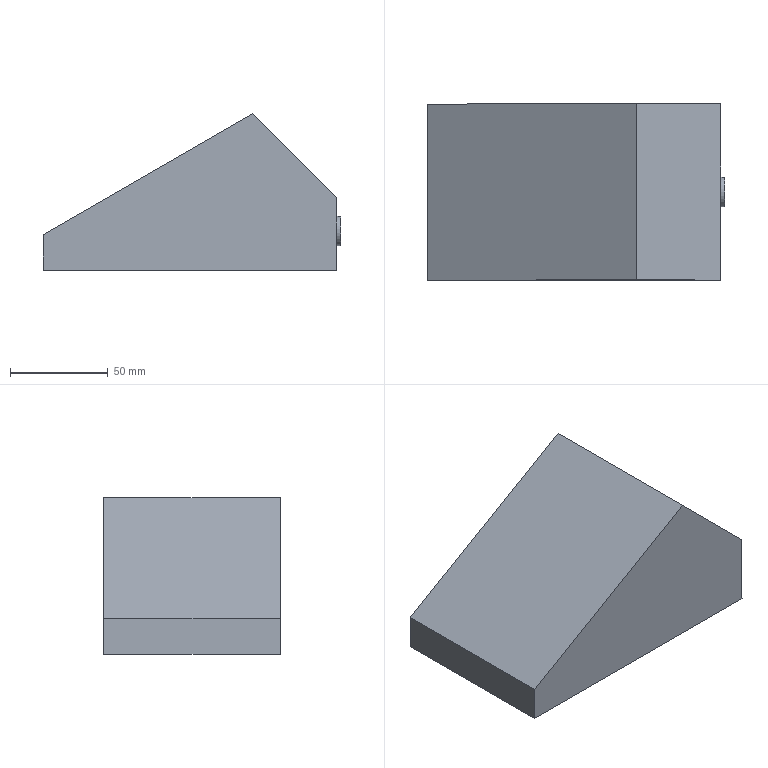Part | NX | features solid 2 | 1 solid | 9 faces | box 152 x 90 x 80 mm | volume 699695 mm3 | plane 8 | cylinder 1 | commonest cylinder face diameters 15 x1
STEP:
#1=CARTESIAN_POINT('',(833.,-335.,-236.776));
#2=VERTEX_POINT('',#1);
#3=CARTESIAN_POINT('',(833.,-335.,-255.));
#4=VERTEX_POINT('',#3);
#5=CARTESIAN_POINT('',(833.,-335.,-236.776));
#6=CARTESIAN_POINT('',(833.,-335.,-242.851));
#7=CARTESIAN_POINT('',(833.,-335.,-248.925));
#8=CARTESIAN_POINT('',(833.,-335.,-255.));
#9=B_SPLINE_CURVE_WITH_KNOTS('',3,(#5,#6,#7,#8),.UNSPECIFIED.,.F.,.F.,(4,4),(0.7722,1.),.UNSPECIFIED.);
#10=EDGE_CURVE('',#2,#4,#9,.T.);
#11=ORIENTED_EDGE('',*,*,#10,.F.);
#12=CARTESIAN_POINT('',(940.,-335.,-175.));
#13=VERTEX_POINT('',#12);
#14=CARTESIAN_POINT('',(916.,-335.,-188.856));
#15=DIRECTION('',(0.866,-0.000000076,0.5));
#16=VECTOR('',#15,1000.);
#17=LINE('',#14,#16);
#18=EDGE_CURVE('',#2,#13,#17,.T.);
#19=ORIENTED_EDGE('',*,*,#18,.T.);
#20=CARTESIAN_POINT('',(983.,-335.,-218.));
#21=VERTEX_POINT('',#20);
#22=CARTESIAN_POINT('',(924.,-335.,-159.));
#23=DIRECTION('',(0.7071,0.000000128,-0.7071));
#24=VECTOR('',#23,1000.);
#25=LINE('',#22,#24);
#26=EDGE_CURVE('',#13,#21,#25,.T.);
#27=ORIENTED_EDGE('',*,*,#26,.T.);
#28=CARTESIAN_POINT('',(983.,-335.,-255.));
#29=VERTEX_POINT('',#28);
#30=CARTESIAN_POINT('',(983.,-335.,-255.));
#31=CARTESIAN_POINT('',(983.,-335.,-242.666));
#32=CARTESIAN_POINT('',(983.,-335.,-230.333));
#33=CARTESIAN_POINT('',(983.,-335.,-218.));
#34=B_SPLINE_CURVE_WITH_KNOTS('',3,(#30,#31,#32,#33),.UNSPECIFIED.,.F.,.F.,(4,4),(0.,0.4625),.UNSPECIFIED.);
#35=EDGE_CURVE('',#21,#29,#34,.F.);
#36=ORIENTED_EDGE('',*,*,#35,.T.);
#37=CARTESIAN_POINT('',(833.,-335.,-255.));
#38=CARTESIAN_POINT('',(883.,-335.,-255.));
#39=CARTESIAN_POINT('',(933.,-335.,-255.));
#40=CARTESIAN_POINT('',(983.,-335.,-255.));
#41=B_SPLINE_CURVE_WITH_KNOTS('',3,(#37,#38,#39,#40),.UNSPECIFIED.,.F.,.F.,(4,4),(0.,1.),.UNSPECIFIED.);
#42=EDGE_CURVE('',#4,#29,#41,.T.);
#43=ORIENTED_EDGE('',*,*,#42,.F.);
#44=EDGE_LOOP('',(#11,#19,#27,#36,#43));
#45=FACE_BOUND('',#44,.T.);
#46=CARTESIAN_POINT('',(908.,-335.,-175.));
#47=DIRECTION('',(-0.000000011,1.,0.00000017));
#48=DIRECTION('',(-0.000000341,-0.00000017,1.));
#49=AXIS2_PLACEMENT_3D('',#46,#47,#48);
#50=PLANE('',#49);
#51=ADVANCED_FACE('',(#45),#50,.T.);
#52=CARTESIAN_POINT('',(983.,-379.998,-242.5));
#53=VERTEX_POINT('',#52);
#54=CARTESIAN_POINT('',(983.,-379.998,-235.));
#55=DIRECTION('',(1.,0.000000011,0.000000341));
#56=DIRECTION('',(0.000000341,0.00000017,-1.));
#57=AXIS2_PLACEMENT_3D('',#54,#55,#56);
#58=CIRCLE('',#57,7.5);
#59=EDGE_CURVE('',#53,#53,#58,.T.);
#60=ORIENTED_EDGE('',*,*,#59,.F.);
#61=EDGE_LOOP('',(#60));
#62=FACE_BOUND('',#61,.T.);
#63=ORIENTED_EDGE('',*,*,#35,.F.);
#64=CARTESIAN_POINT('',(983.,-425.,-218.));
#65=VERTEX_POINT('',#64);
#66=CARTESIAN_POINT('',(983.,-425.,-218.));
#67=DIRECTION('',(0.000000011,-1.,-0.00000017));
#68=VECTOR('',#67,1000.);
#69=LINE('',#66,#68);
#70=EDGE_CURVE('',#21,#65,#69,.T.);
#71=ORIENTED_EDGE('',*,*,#70,.T.);
#72=CARTESIAN_POINT('',(983.,-425.,-255.));
#73=VERTEX_POINT('',#72);
#74=CARTESIAN_POINT('',(983.,-425.,-255.));
#75=CARTESIAN_POINT('',(983.,-425.,-242.666));
#76=CARTESIAN_POINT('',(983.,-425.,-230.333));
#77=CARTESIAN_POINT('',(983.,-425.,-218.));
#78=B_SPLINE_CURVE_WITH_KNOTS('',3,(#74,#75,#76,#77),.UNSPECIFIED.,.F.,.F.,(4,4),(0.,0.4625),.UNSPECIFIED.);
#79=EDGE_CURVE('',#65,#73,#78,.F.);
#80=ORIENTED_EDGE('',*,*,#79,.T.);
#81=CARTESIAN_POINT('',(983.,-335.,-255.));
#82=CARTESIAN_POINT('',(983.,-365.,-255.));
#83=CARTESIAN_POINT('',(983.,-395.,-255.));
#84=CARTESIAN_POINT('',(983.,-425.,-255.));
#85=B_SPLINE_CURVE_WITH_KNOTS('',3,(#81,#82,#83,#84),.UNSPECIFIED.,.F.,.F.,(4,4),(0.,1.),.UNSPECIFIED.);
#86=EDGE_CURVE('',#29,#73,#85,.T.);
#87=ORIENTED_EDGE('',*,*,#86,.F.);
#88=EDGE_LOOP('',(#63,#71,#80,#87));
#89=FACE_BOUND('',#88,.T.);
#90=CARTESIAN_POINT('',(983.,-380.,-175.));
#91=DIRECTION('',(1.,0.000000011,0.000000341));
#92=DIRECTION('',(0.000000341,0.00000017,-1.));
#93=AXIS2_PLACEMENT_3D('',#90,#91,#92);
#94=PLANE('',#93);
#95=ADVANCED_FACE('',(#62,#89),#94,.T.);
#96=CARTESIAN_POINT('',(940.,-425.,-175.));
#97=VERTEX_POINT('',#96);
#98=CARTESIAN_POINT('',(924.,-425.,-159.));
#99=DIRECTION('',(-0.7071,-0.000000128,0.7071));
#100=VECTOR('',#99,1000.);
#101=LINE('',#98,#100);
#102=EDGE_CURVE('',#65,#97,#101,.T.);
#103=ORIENTED_EDGE('',*,*,#102,.T.);
#104=CARTESIAN_POINT('',(833.,-425.,-236.776));
#105=VERTEX_POINT('',#104);
#106=CARTESIAN_POINT('',(916.,-425.,-188.856));
#107=DIRECTION('',(-0.866,0.000000076,-0.5));
#108=VECTOR('',#107,1000.);
#109=LINE('',#106,#108);
#110=EDGE_CURVE('',#97,#105,#109,.T.);
#111=ORIENTED_EDGE('',*,*,#110,.T.);
#112=CARTESIAN_POINT('',(833.,-425.,-255.));
#113=VERTEX_POINT('',#112);
#114=CARTESIAN_POINT('',(833.,-425.,-255.));
#115=CARTESIAN_POINT('',(833.,-425.,-248.925));
#116=CARTESIAN_POINT('',(833.,-425.,-242.851));
#117=CARTESIAN_POINT('',(833.,-425.,-236.776));
#118=B_SPLINE_CURVE_WITH_KNOTS('',3,(#114,#115,#116,#117),.UNSPECIFIED.,.F.,.F.,(4,4),(0.,0.2278),.UNSPECIFIED.);
#119=EDGE_CURVE('',#105,#113,#118,.F.);
#120=ORIENTED_EDGE('',*,*,#119,.T.);
#121=CARTESIAN_POINT('',(983.,-425.,-255.));
#122=CARTESIAN_POINT('',(933.,-425.,-255.));
#123=CARTESIAN_POINT('',(883.,-425.,-255.));
#124=CARTESIAN_POINT('',(833.,-425.,-255.));
#125=B_SPLINE_CURVE_WITH_KNOTS('',3,(#121,#122,#123,#124),.UNSPECIFIED.,.F.,.F.,(4,4),(0.,1.),.UNSPECIFIED.);
#126=EDGE_CURVE('',#73,#113,#125,.T.);
#127=ORIENTED_EDGE('',*,*,#126,.F.);
#128=ORIENTED_EDGE('',*,*,#79,.F.);
#129=EDGE_LOOP('',(#103,#111,#120,#127,#128));
#130=FACE_BOUND('',#129,.T.);
#131=CARTESIAN_POINT('',(908.,-425.,-175.));
#132=DIRECTION('',(0.000000011,-1.,-0.00000017));
#133=DIRECTION('',(0.000000341,0.00000017,-1.));
#134=AXIS2_PLACEMENT_3D('',#131,#132,#133);
#135=PLANE('',#134);
#136=ADVANCED_FACE('',(#130),#135,.T.);
#137=ORIENTED_EDGE('',*,*,#119,.F.);
#138=CARTESIAN_POINT('',(833.,-335.,-236.776));
#139=DIRECTION('',(-0.000000011,1.,0.00000017));
#140=VECTOR('',#139,1000.);
#141=LINE('',#138,#140);
#142=EDGE_CURVE('',#105,#2,#141,.T.);
#143=ORIENTED_EDGE('',*,*,#142,.T.);
#144=ORIENTED_EDGE('',*,*,#10,.T.);
#145=CARTESIAN_POINT('',(833.,-425.,-255.));
#146=CARTESIAN_POINT('',(833.,-395.,-255.));
#147=CARTESIAN_POINT('',(833.,-365.,-255.));
#148=CARTESIAN_POINT('',(833.,-335.,-255.));
#149=B_SPLINE_CURVE_WITH_KNOTS('',3,(#145,#146,#147,#148),.UNSPECIFIED.,.F.,.F.,(4,4),(0.,1.),.UNSPECIFIED.);
#150=EDGE_CURVE('',#113,#4,#149,.T.);
#151=ORIENTED_EDGE('',*,*,#150,.F.);
#152=EDGE_LOOP('',(#137,#143,#144,#151));
#153=FACE_BOUND('',#152,.T.);
#154=CARTESIAN_POINT('',(833.,-380.,-175.));
#155=DIRECTION('',(-1.,-0.000000011,-0.000000341));
#156=DIRECTION('',(-0.000000341,-0.00000017,1.));
#157=AXIS2_PLACEMENT_3D('',#154,#155,#156);
#158=PLANE('',#157);
#159=ADVANCED_FACE('',(#153),#158,.T.);
#160=ORIENTED_EDGE('',*,*,#42,.T.);
#161=ORIENTED_EDGE('',*,*,#86,.T.);
#162=ORIENTED_EDGE('',*,*,#126,.T.);
#163=ORIENTED_EDGE('',*,*,#150,.T.);
#164=EDGE_LOOP('',(#160,#161,#162,#163));
#165=FACE_BOUND('',#164,.T.);
#166=CARTESIAN_POINT('',(908.,-380.,-255.));
#167=DIRECTION('',(0.000000341,0.00000017,-1.));
#168=DIRECTION('',(0.000000011,-1.,-0.00000017));
#169=AXIS2_PLACEMENT_3D('',#166,#167,#168);
#170=PLANE('',#169);
#171=ADVANCED_FACE('',(#165),#170,.T.);
#172=ORIENTED_EDGE('',*,*,#26,.F.);
#173=CARTESIAN_POINT('',(940.,-335.,-175.));
#174=DIRECTION('',(-0.000000011,1.,0.00000017));
#175=VECTOR('',#174,1000.);
#176=LINE('',#173,#175);
#177=EDGE_CURVE('',#97,#13,#176,.T.);
#178=ORIENTED_EDGE('',*,*,#177,.F.);
#179=ORIENTED_EDGE('',*,*,#102,.F.);
#180=ORIENTED_EDGE('',*,*,#70,.F.);
#181=EDGE_LOOP('',(#172,#178,#179,#180));
#182=FACE_BOUND('',#181,.T.);
#183=CARTESIAN_POINT('',(983.,-380.,-218.));
#184=DIRECTION('',(0.7071,-0.000000113,0.7071));
#185=DIRECTION('',(0.7071,0.000000128,-0.7071));
#186=AXIS2_PLACEMENT_3D('',#183,#184,#185);
#187=PLANE('',#186);
#188=ADVANCED_FACE('',(#182),#187,.T.);
#189=ORIENTED_EDGE('',*,*,#110,.F.);
#190=ORIENTED_EDGE('',*,*,#177,.T.);
#191=ORIENTED_EDGE('',*,*,#18,.F.);
#192=ORIENTED_EDGE('',*,*,#142,.F.);
#193=EDGE_LOOP('',(#189,#190,#191,#192));
#194=FACE_BOUND('',#193,.T.);
#195=CARTESIAN_POINT('',(833.,-380.,-236.776));
#196=DIRECTION('',(-0.5,-0.000000153,0.866));
#197=DIRECTION('',(0.866,-0.000000076,0.5));
#198=AXIS2_PLACEMENT_3D('',#195,#196,#197);
#199=PLANE('',#198);
#200=ADVANCED_FACE('',(#194),#199,.T.);
#201=CARTESIAN_POINT('',(985.,-379.998,-242.5));
#202=VERTEX_POINT('',#201);
#203=CARTESIAN_POINT('',(985.,-379.998,-235.));
#204=DIRECTION('',(1.,0.000000011,0.000000341));
#205=DIRECTION('',(0.000000341,0.00000017,-1.));
#206=AXIS2_PLACEMENT_3D('',#203,#204,#205);
#207=CIRCLE('',#206,7.5);
#208=EDGE_CURVE('',#202,#202,#207,.T.);
#209=ORIENTED_EDGE('',*,*,#208,.T.);
#210=EDGE_LOOP('',(#209));
#211=FACE_BOUND('',#210,.T.);
#212=CARTESIAN_POINT('',(985.,-379.998,-235.));
#213=DIRECTION('',(1.,0.000000011,0.000000341));
#214=DIRECTION('',(0.000000341,0.00000017,-1.));
#215=AXIS2_PLACEMENT_3D('',#212,#213,#214);
#216=PLANE('',#215);
#217=ADVANCED_FACE('',(#211),#216,.T.);
#218=ORIENTED_EDGE('',*,*,#208,.F.);
#219=EDGE_LOOP('',(#218));
#220=FACE_BOUND('',#219,.T.);
#221=ORIENTED_EDGE('',*,*,#59,.T.);
#222=EDGE_LOOP('',(#221));
#223=FACE_BOUND('',#222,.T.);
#224=CARTESIAN_POINT('',(983.,-379.998,-235.));
#225=DIRECTION('',(1.,0.000000011,0.000000341));
#226=DIRECTION('',(0.000000341,0.00000017,-1.));
#227=AXIS2_PLACEMENT_3D('',#224,#225,#226);
#228=CYLINDRICAL_SURFACE('',#227,7.5);
#229=ADVANCED_FACE('',(#220,#223),#228,.T.);
#230=CLOSED_SHELL('',(#51,#95,#136,#159,#171,#188,#200,#217,#229));
#231=MANIFOLD_SOLID_BREP('',#230);
#232=(LENGTH_UNIT()NAMED_UNIT(*)SI_UNIT(.MILLI.,.METRE.));
#233=UNCERTAINTY_MEASURE_WITH_UNIT(LENGTH_MEASURE(0.0508),#232,'','');
#234=(NAMED_UNIT(*)PLANE_ANGLE_UNIT()SI_UNIT($,.RADIAN.));
#235=(NAMED_UNIT(*)SI_UNIT($,.STERADIAN.)SOLID_ANGLE_UNIT());
#236=(GEOMETRIC_REPRESENTATION_CONTEXT(3)GLOBAL_UNCERTAINTY_ASSIGNED_CONTEXT((#233))GLOBAL_UNIT_ASSIGNED_CONTEXT((#232,#234,#235))REPRESENTATION_CONTEXT('',''));
#237=ADVANCED_BREP_SHAPE_REPRESENTATION('',(#231),#236);